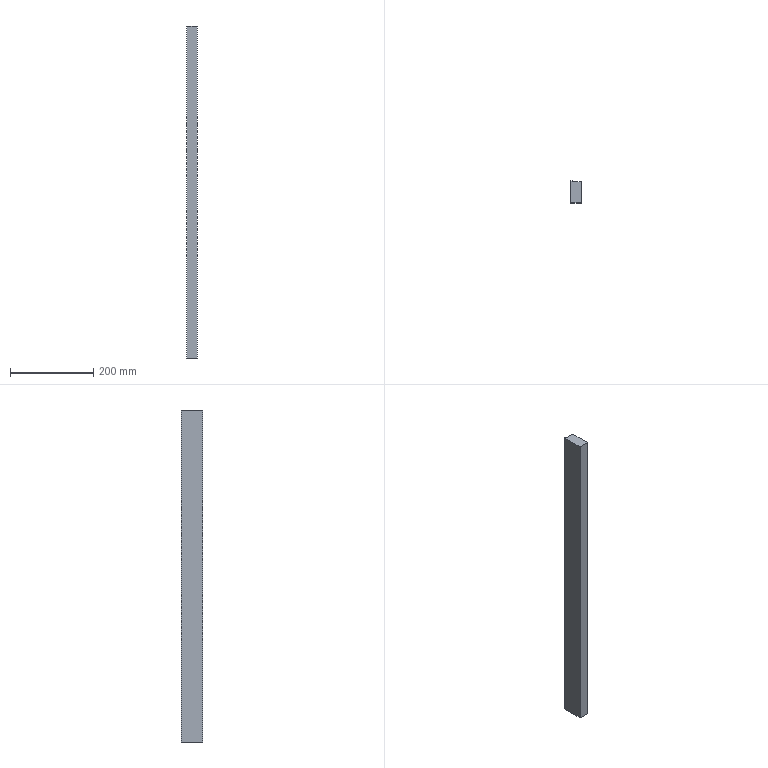Part | SolidWorks | features Extrusion 1 | 1 solid | 8 faces | box 25 x 53 x 800 mm | volume 1009600 mm3 | plane 8
STEP:
#1=CARTESIAN_POINT('',(-10.,-12.5,-800.));
#2=VERTEX_POINT('',#1);
#3=CARTESIAN_POINT('',(-10.,-15.5,-800.));
#4=VERTEX_POINT('',#3);
#5=CARTESIAN_POINT('',(-10.,-15.5,-800.));
#6=DIRECTION('',(0.,-1.,0.));
#7=VECTOR('',#6,1000.);
#8=LINE('',#5,#7);
#9=EDGE_CURVE('',#2,#4,#8,.T.);
#10=ORIENTED_EDGE('',*,*,#9,.F.);
#11=CARTESIAN_POINT('',(-10.,-12.5,0.));
#12=VERTEX_POINT('',#11);
#13=CARTESIAN_POINT('',(-10.,-12.5,-858.6));
#14=DIRECTION('',(0.,0.,1.));
#15=VECTOR('',#14,1000.);
#16=LINE('',#13,#15);
#17=EDGE_CURVE('',#2,#12,#16,.T.);
#18=ORIENTED_EDGE('',*,*,#17,.T.);
#19=CARTESIAN_POINT('',(-10.,-15.5,0.));
#20=VERTEX_POINT('',#19);
#21=CARTESIAN_POINT('',(-10.,-15.5,0.));
#22=DIRECTION('',(0.,1.,0.));
#23=VECTOR('',#22,1000.);
#24=LINE('',#21,#23);
#25=EDGE_CURVE('',#20,#12,#24,.T.);
#26=ORIENTED_EDGE('',*,*,#25,.F.);
#27=CARTESIAN_POINT('',(-10.,-15.5,-858.6));
#28=DIRECTION('',(0.,0.,1.));
#29=VECTOR('',#28,1000.);
#30=LINE('',#27,#29);
#31=EDGE_CURVE('',#4,#20,#30,.T.);
#32=ORIENTED_EDGE('',*,*,#31,.F.);
#33=EDGE_LOOP('',(#10,#18,#26,#32));
#34=FACE_OUTER_BOUND('',#33,.T.);
#35=CARTESIAN_POINT('',(-10.,-15.5,-858.6));
#36=DIRECTION('',(1.,0.,0.));
#37=DIRECTION('',(0.,0.,-1.));
#38=AXIS2_PLACEMENT_3D('',#35,#36,#37);
#39=PLANE('',#38);
#40=ADVANCED_FACE('',(#34),#39,.T.);
#41=CARTESIAN_POINT('',(11.,-15.5,-800.));
#42=VERTEX_POINT('',#41);
#43=CARTESIAN_POINT('',(11.,-15.5,-800.));
#44=DIRECTION('',(1.,0.,0.));
#45=VECTOR('',#44,1000.);
#46=LINE('',#43,#45);
#47=EDGE_CURVE('',#4,#42,#46,.T.);
#48=ORIENTED_EDGE('',*,*,#47,.F.);
#49=ORIENTED_EDGE('',*,*,#31,.T.);
#50=CARTESIAN_POINT('',(11.,-15.5,0.));
#51=VERTEX_POINT('',#50);
#52=CARTESIAN_POINT('',(11.,-15.5,0.));
#53=DIRECTION('',(-1.,0.,0.));
#54=VECTOR('',#53,1000.);
#55=LINE('',#52,#54);
#56=EDGE_CURVE('',#51,#20,#55,.T.);
#57=ORIENTED_EDGE('',*,*,#56,.F.);
#58=CARTESIAN_POINT('',(11.,-15.5,-858.6));
#59=DIRECTION('',(0.,0.,1.));
#60=VECTOR('',#59,1000.);
#61=LINE('',#58,#60);
#62=EDGE_CURVE('',#42,#51,#61,.T.);
#63=ORIENTED_EDGE('',*,*,#62,.F.);
#64=EDGE_LOOP('',(#48,#49,#57,#63));
#65=FACE_OUTER_BOUND('',#64,.T.);
#66=CARTESIAN_POINT('',(11.,-15.5,-858.6));
#67=DIRECTION('',(0.,1.,0.));
#68=DIRECTION('',(-1.,0.,0.));
#69=AXIS2_PLACEMENT_3D('',#66,#67,#68);
#70=PLANE('',#69);
#71=ADVANCED_FACE('',(#65),#70,.T.);
#72=CARTESIAN_POINT('',(11.,-65.5,-800.));
#73=VERTEX_POINT('',#72);
#74=CARTESIAN_POINT('',(11.,-65.5,-800.));
#75=DIRECTION('',(0.,-1.,0.));
#76=VECTOR('',#75,1000.);
#77=LINE('',#74,#76);
#78=EDGE_CURVE('',#42,#73,#77,.T.);
#79=ORIENTED_EDGE('',*,*,#78,.F.);
#80=ORIENTED_EDGE('',*,*,#62,.T.);
#81=CARTESIAN_POINT('',(11.,-65.5,0.));
#82=VERTEX_POINT('',#81);
#83=CARTESIAN_POINT('',(11.,-65.5,0.));
#84=DIRECTION('',(0.,1.,0.));
#85=VECTOR('',#84,1000.);
#86=LINE('',#83,#85);
#87=EDGE_CURVE('',#82,#51,#86,.T.);
#88=ORIENTED_EDGE('',*,*,#87,.F.);
#89=CARTESIAN_POINT('',(11.,-65.5,-858.6));
#90=DIRECTION('',(0.,0.,1.));
#91=VECTOR('',#90,1000.);
#92=LINE('',#89,#91);
#93=EDGE_CURVE('',#73,#82,#92,.T.);
#94=ORIENTED_EDGE('',*,*,#93,.F.);
#95=EDGE_LOOP('',(#79,#80,#88,#94));
#96=FACE_OUTER_BOUND('',#95,.T.);
#97=CARTESIAN_POINT('',(11.,-65.5,-858.6));
#98=DIRECTION('',(1.,0.,0.));
#99=DIRECTION('',(0.,1.,0.));
#100=AXIS2_PLACEMENT_3D('',#97,#98,#99);
#101=PLANE('',#100);
#102=ADVANCED_FACE('',(#96),#101,.T.);
#103=CARTESIAN_POINT('',(-14.,-65.5,-800.));
#104=VERTEX_POINT('',#103);
#105=CARTESIAN_POINT('',(-14.,-65.5,-800.));
#106=DIRECTION('',(-1.,0.,0.));
#107=VECTOR('',#106,1000.);
#108=LINE('',#105,#107);
#109=EDGE_CURVE('',#73,#104,#108,.T.);
#110=ORIENTED_EDGE('',*,*,#109,.F.);
#111=ORIENTED_EDGE('',*,*,#93,.T.);
#112=CARTESIAN_POINT('',(-14.,-65.5,0.));
#113=VERTEX_POINT('',#112);
#114=CARTESIAN_POINT('',(-14.,-65.5,0.));
#115=DIRECTION('',(1.,0.,0.));
#116=VECTOR('',#115,1000.);
#117=LINE('',#114,#116);
#118=EDGE_CURVE('',#113,#82,#117,.T.);
#119=ORIENTED_EDGE('',*,*,#118,.F.);
#120=CARTESIAN_POINT('',(-14.,-65.5,-858.6));
#121=DIRECTION('',(0.,0.,1.));
#122=VECTOR('',#121,1000.);
#123=LINE('',#120,#122);
#124=EDGE_CURVE('',#104,#113,#123,.T.);
#125=ORIENTED_EDGE('',*,*,#124,.F.);
#126=EDGE_LOOP('',(#110,#111,#119,#125));
#127=FACE_OUTER_BOUND('',#126,.T.);
#128=CARTESIAN_POINT('',(-14.,-65.5,-858.6));
#129=DIRECTION('',(0.,-1.,0.));
#130=DIRECTION('',(0.,0.,-1.));
#131=AXIS2_PLACEMENT_3D('',#128,#129,#130);
#132=PLANE('',#131);
#133=ADVANCED_FACE('',(#127),#132,.T.);
#134=CARTESIAN_POINT('',(-14.,-12.5,-800.));
#135=VERTEX_POINT('',#134);
#136=CARTESIAN_POINT('',(-14.,-12.5,-800.));
#137=DIRECTION('',(0.,1.,0.));
#138=VECTOR('',#137,1000.);
#139=LINE('',#136,#138);
#140=EDGE_CURVE('',#104,#135,#139,.T.);
#141=ORIENTED_EDGE('',*,*,#140,.F.);
#142=ORIENTED_EDGE('',*,*,#124,.T.);
#143=CARTESIAN_POINT('',(-14.,-12.5,0.));
#144=VERTEX_POINT('',#143);
#145=CARTESIAN_POINT('',(-14.,-12.5,0.));
#146=DIRECTION('',(0.,-1.,0.));
#147=VECTOR('',#146,1000.);
#148=LINE('',#145,#147);
#149=EDGE_CURVE('',#144,#113,#148,.T.);
#150=ORIENTED_EDGE('',*,*,#149,.F.);
#151=CARTESIAN_POINT('',(-14.,-12.5,-858.6));
#152=DIRECTION('',(0.,0.,1.));
#153=VECTOR('',#152,1000.);
#154=LINE('',#151,#153);
#155=EDGE_CURVE('',#135,#144,#154,.T.);
#156=ORIENTED_EDGE('',*,*,#155,.F.);
#157=EDGE_LOOP('',(#141,#142,#150,#156));
#158=FACE_OUTER_BOUND('',#157,.T.);
#159=CARTESIAN_POINT('',(-14.,-12.5,-858.6));
#160=DIRECTION('',(-1.,0.,0.));
#161=DIRECTION('',(0.,-1.,0.));
#162=AXIS2_PLACEMENT_3D('',#159,#160,#161);
#163=PLANE('',#162);
#164=ADVANCED_FACE('',(#158),#163,.T.);
#165=CARTESIAN_POINT('',(-10.,-12.5,-800.));
#166=DIRECTION('',(1.,0.,0.));
#167=VECTOR('',#166,1000.);
#168=LINE('',#165,#167);
#169=EDGE_CURVE('',#135,#2,#168,.T.);
#170=ORIENTED_EDGE('',*,*,#169,.F.);
#171=ORIENTED_EDGE('',*,*,#155,.T.);
#172=CARTESIAN_POINT('',(-10.,-12.5,0.));
#173=DIRECTION('',(-1.,0.,0.));
#174=VECTOR('',#173,1000.);
#175=LINE('',#172,#174);
#176=EDGE_CURVE('',#12,#144,#175,.T.);
#177=ORIENTED_EDGE('',*,*,#176,.F.);
#178=ORIENTED_EDGE('',*,*,#17,.F.);
#179=EDGE_LOOP('',(#170,#171,#177,#178));
#180=FACE_OUTER_BOUND('',#179,.T.);
#181=CARTESIAN_POINT('',(-10.,-12.5,-858.6));
#182=DIRECTION('',(0.,1.,0.));
#183=DIRECTION('',(0.,0.,1.));
#184=AXIS2_PLACEMENT_3D('',#181,#182,#183);
#185=PLANE('',#184);
#186=ADVANCED_FACE('',(#180),#185,.T.);
#187=ORIENTED_EDGE('',*,*,#25,.T.);
#188=ORIENTED_EDGE('',*,*,#176,.T.);
#189=ORIENTED_EDGE('',*,*,#149,.T.);
#190=ORIENTED_EDGE('',*,*,#118,.T.);
#191=ORIENTED_EDGE('',*,*,#87,.T.);
#192=ORIENTED_EDGE('',*,*,#56,.T.);
#193=EDGE_LOOP('',(#187,#188,#189,#190,#191,#192));
#194=FACE_OUTER_BOUND('',#193,.T.);
#195=CARTESIAN_POINT('',(0.,0.,0.));
#196=DIRECTION('',(0.,0.,1.));
#197=DIRECTION('',(1.,0.,0.));
#198=AXIS2_PLACEMENT_3D('',#195,#196,#197);
#199=PLANE('',#198);
#200=ADVANCED_FACE('',(#194),#199,.T.);
#201=ORIENTED_EDGE('',*,*,#9,.T.);
#202=ORIENTED_EDGE('',*,*,#47,.T.);
#203=ORIENTED_EDGE('',*,*,#78,.T.);
#204=ORIENTED_EDGE('',*,*,#109,.T.);
#205=ORIENTED_EDGE('',*,*,#140,.T.);
#206=ORIENTED_EDGE('',*,*,#169,.T.);
#207=EDGE_LOOP('',(#201,#202,#203,#204,#205,#206));
#208=FACE_OUTER_BOUND('',#207,.T.);
#209=CARTESIAN_POINT('',(9.5,-10.283,-800.));
#210=DIRECTION('',(0.,0.,1.));
#211=DIRECTION('',(1.,0.,0.));
#212=AXIS2_PLACEMENT_3D('',#209,#210,#211);
#213=PLANE('',#212);
#214=ADVANCED_FACE('',(#208),#213,.F.);
#215=CLOSED_SHELL('',(#40,#71,#102,#133,#164,#186,#200,#214));
#216=MANIFOLD_SOLID_BREP('',#215);
#217=CARTESIAN_POINT('',(0.,0.,0.));
#218=DIRECTION('',(0.,0.,1.));
#219=DIRECTION('',(1.,0.,0.));
#220=AXIS2_PLACEMENT_3D('',#217,#218,#219);
#221=(LENGTH_UNIT()NAMED_UNIT(*)SI_UNIT(.MILLI.,.METRE.));
#222=UNCERTAINTY_MEASURE_WITH_UNIT(LENGTH_MEASURE(0.00001),#221,'','');
#223=(NAMED_UNIT(*)PLANE_ANGLE_UNIT()SI_UNIT($,.RADIAN.));
#224=(NAMED_UNIT(*)SI_UNIT($,.STERADIAN.)SOLID_ANGLE_UNIT());
#225=(GEOMETRIC_REPRESENTATION_CONTEXT(3)GLOBAL_UNCERTAINTY_ASSIGNED_CONTEXT((#222))GLOBAL_UNIT_ASSIGNED_CONTEXT((#221,#223,#224))REPRESENTATION_CONTEXT('',''));
#226=ADVANCED_BREP_SHAPE_REPRESENTATION('',(#216,#220),#225);